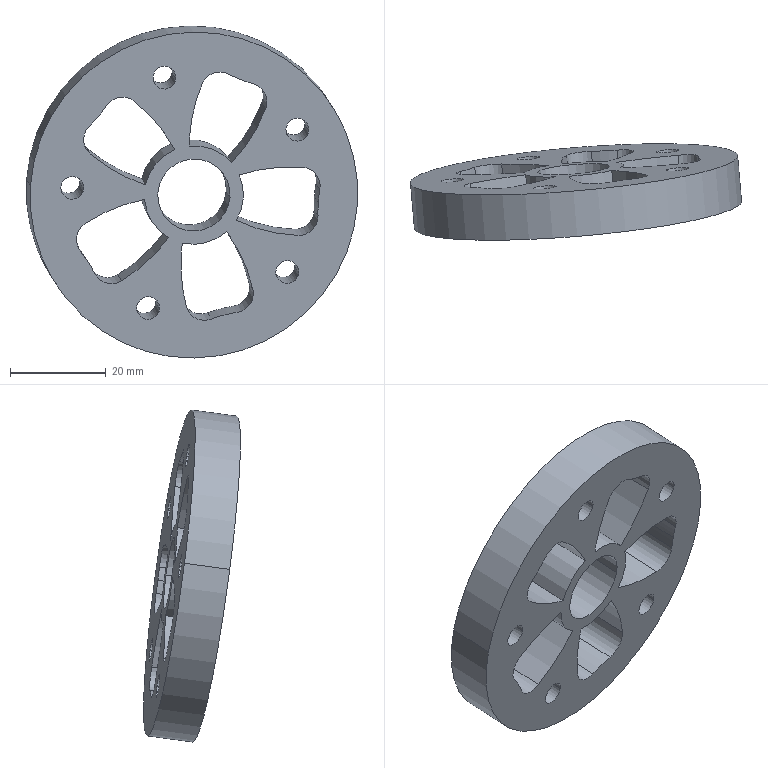Part | SolidWorks | features SplitBody 1 | 1 solid | 51 faces | box 69.36 x 20.284 x 69.466 mm | volume 22930 mm3 | cylinder 49 | plane 2 | commonest cylinder face diameters 68.8 x14 8 x12 4.8 x10 56 x6 20.8 x5 15.2 x2